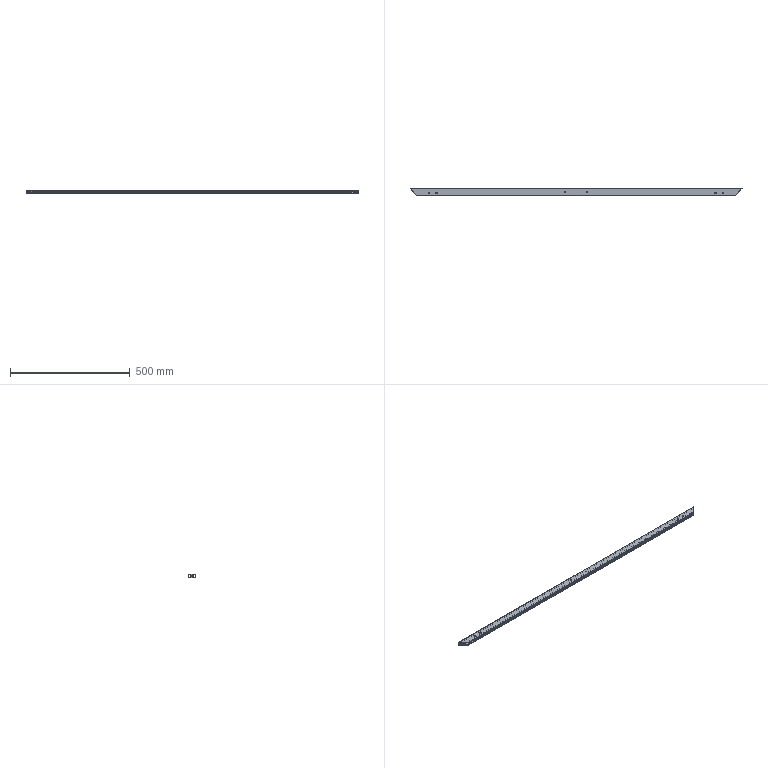Part | SolidWorks | features HoleWzd 2, 3DProfileFeature 1, ICE 1, WeldMemberFeat 1, WeldmentFeature 1 | 1 solid | 52 faces | box 1386 x 30 x 15 mm | volume 332572 mm3 | cylinder 32 | plane 20 | commonest cylinder face diameters 5 x14 6.8 x8 12 x6 3 x4